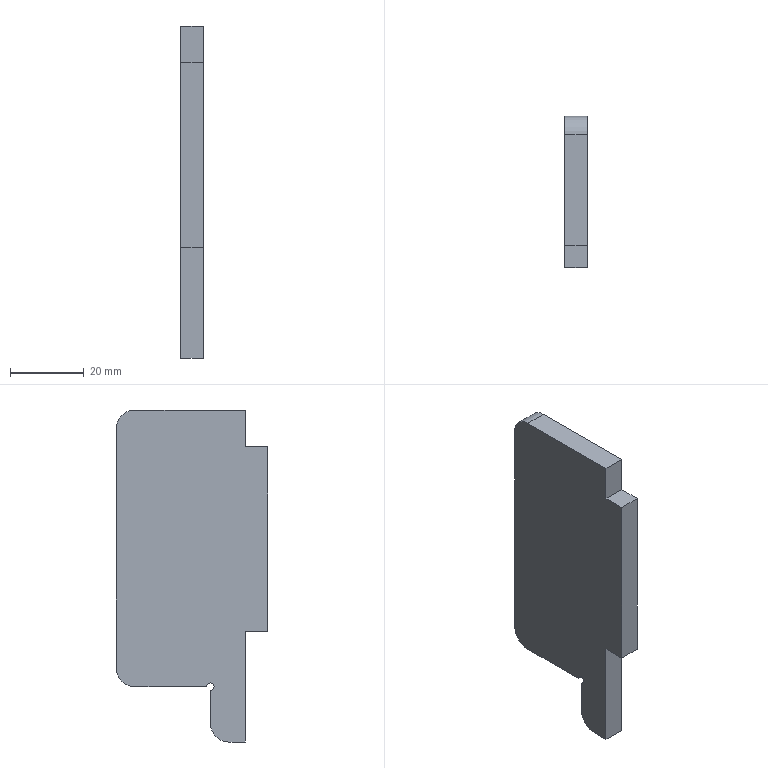Part | SolidWorks | features FlatPattern 1, SMBaseFlange 1, SheetMetal 1 | 1 solid | 16 faces | box 6 x 41 x 90 mm | volume 18294 mm3 | plane 12 | cylinder 4 | commonest cylinder face diameters 10 x3 2 x1
STEP:
#1=CARTESIAN_POINT('',(0.,0.,0.));
#2=VERTEX_POINT('',#1);
#3=CARTESIAN_POINT('',(0.,4.5,0.));
#4=VERTEX_POINT('',#3);
#5=CARTESIAN_POINT('',(0.,4.5,0.));
#6=DIRECTION('',(0.,1.,0.));
#7=VECTOR('',#6,1000.);
#8=LINE('',#5,#7);
#9=EDGE_CURVE('',#2,#4,#8,.T.);
#10=ORIENTED_EDGE('',*,*,#9,.F.);
#11=CARTESIAN_POINT('',(-6.,0.,0.));
#12=VERTEX_POINT('',#11);
#13=CARTESIAN_POINT('',(-6.,0.,0.));
#14=DIRECTION('',(1.,0.,0.));
#15=VECTOR('',#14,1000.);
#16=LINE('',#13,#15);
#17=EDGE_CURVE('',#12,#2,#16,.T.);
#18=ORIENTED_EDGE('',*,*,#17,.F.);
#19=CARTESIAN_POINT('',(-6.,4.5,0.));
#20=VERTEX_POINT('',#19);
#21=CARTESIAN_POINT('',(-6.,4.5,0.));
#22=DIRECTION('',(0.,1.,0.));
#23=VECTOR('',#22,1000.);
#24=LINE('',#21,#23);
#25=EDGE_CURVE('',#12,#20,#24,.T.);
#26=ORIENTED_EDGE('',*,*,#25,.T.);
#27=CARTESIAN_POINT('',(-6.,4.5,0.));
#28=DIRECTION('',(1.,0.,0.));
#29=VECTOR('',#28,1000.);
#30=LINE('',#27,#29);
#31=EDGE_CURVE('',#20,#4,#30,.T.);
#32=ORIENTED_EDGE('',*,*,#31,.T.);
#33=EDGE_LOOP('',(#10,#18,#26,#32));
#34=FACE_OUTER_BOUND('',#33,.T.);
#35=CARTESIAN_POINT('',(-6.,4.5,0.));
#36=DIRECTION('',(0.,0.,-1.));
#37=DIRECTION('',(-1.,0.,0.));
#38=AXIS2_PLACEMENT_3D('',#35,#36,#37);
#39=PLANE('',#38);
#40=ADVANCED_FACE('',(#34),#39,.T.);
#41=CARTESIAN_POINT('',(0.,0.,30.));
#42=VERTEX_POINT('',#41);
#43=CARTESIAN_POINT('',(0.,0.,0.));
#44=DIRECTION('',(0.,0.,-1.));
#45=VECTOR('',#44,1000.);
#46=LINE('',#43,#45);
#47=EDGE_CURVE('',#42,#2,#46,.T.);
#48=ORIENTED_EDGE('',*,*,#47,.F.);
#49=CARTESIAN_POINT('',(-6.,0.,30.));
#50=VERTEX_POINT('',#49);
#51=CARTESIAN_POINT('',(-6.,0.,30.));
#52=DIRECTION('',(1.,0.,0.));
#53=VECTOR('',#52,1000.);
#54=LINE('',#51,#53);
#55=EDGE_CURVE('',#50,#42,#54,.T.);
#56=ORIENTED_EDGE('',*,*,#55,.F.);
#57=CARTESIAN_POINT('',(-6.,0.,0.));
#58=DIRECTION('',(0.,0.,-1.));
#59=VECTOR('',#58,1000.);
#60=LINE('',#57,#59);
#61=EDGE_CURVE('',#50,#12,#60,.T.);
#62=ORIENTED_EDGE('',*,*,#61,.T.);
#63=ORIENTED_EDGE('',*,*,#17,.T.);
#64=EDGE_LOOP('',(#48,#56,#62,#63));
#65=FACE_OUTER_BOUND('',#64,.T.);
#66=CARTESIAN_POINT('',(-6.,0.,0.));
#67=DIRECTION('',(0.,-1.,0.));
#68=DIRECTION('',(0.,0.,-1.));
#69=AXIS2_PLACEMENT_3D('',#66,#67,#68);
#70=PLANE('',#69);
#71=ADVANCED_FACE('',(#65),#70,.T.);
#72=CARTESIAN_POINT('',(0.,-6.,30.));
#73=VERTEX_POINT('',#72);
#74=CARTESIAN_POINT('',(0.,-6.,30.));
#75=DIRECTION('',(0.,1.,0.));
#76=VECTOR('',#75,1000.);
#77=LINE('',#74,#76);
#78=EDGE_CURVE('',#73,#42,#77,.T.);
#79=ORIENTED_EDGE('',*,*,#78,.F.);
#80=CARTESIAN_POINT('',(-6.,-6.,30.));
#81=VERTEX_POINT('',#80);
#82=CARTESIAN_POINT('',(-6.,-6.,30.));
#83=DIRECTION('',(1.,0.,0.));
#84=VECTOR('',#83,1000.);
#85=LINE('',#82,#84);
#86=EDGE_CURVE('',#81,#73,#85,.T.);
#87=ORIENTED_EDGE('',*,*,#86,.F.);
#88=CARTESIAN_POINT('',(-6.,-6.,30.));
#89=DIRECTION('',(0.,1.,0.));
#90=VECTOR('',#89,1000.);
#91=LINE('',#88,#90);
#92=EDGE_CURVE('',#81,#50,#91,.T.);
#93=ORIENTED_EDGE('',*,*,#92,.T.);
#94=ORIENTED_EDGE('',*,*,#55,.T.);
#95=EDGE_LOOP('',(#79,#87,#93,#94));
#96=FACE_OUTER_BOUND('',#95,.T.);
#97=CARTESIAN_POINT('',(-6.,-6.,30.));
#98=DIRECTION('',(0.,0.,-1.));
#99=DIRECTION('',(-1.,0.,0.));
#100=AXIS2_PLACEMENT_3D('',#97,#98,#99);
#101=PLANE('',#100);
#102=ADVANCED_FACE('',(#96),#101,.T.);
#103=CARTESIAN_POINT('',(0.,-6.,80.));
#104=VERTEX_POINT('',#103);
#105=CARTESIAN_POINT('',(0.,-6.,80.));
#106=DIRECTION('',(0.,0.,-1.));
#107=VECTOR('',#106,1000.);
#108=LINE('',#105,#107);
#109=EDGE_CURVE('',#104,#73,#108,.T.);
#110=ORIENTED_EDGE('',*,*,#109,.F.);
#111=CARTESIAN_POINT('',(-6.,-6.,80.));
#112=VERTEX_POINT('',#111);
#113=CARTESIAN_POINT('',(-6.,-6.,80.));
#114=DIRECTION('',(1.,0.,0.));
#115=VECTOR('',#114,1000.);
#116=LINE('',#113,#115);
#117=EDGE_CURVE('',#112,#104,#116,.T.);
#118=ORIENTED_EDGE('',*,*,#117,.F.);
#119=CARTESIAN_POINT('',(-6.,-6.,80.));
#120=DIRECTION('',(0.,0.,-1.));
#121=VECTOR('',#120,1000.);
#122=LINE('',#119,#121);
#123=EDGE_CURVE('',#112,#81,#122,.T.);
#124=ORIENTED_EDGE('',*,*,#123,.T.);
#125=ORIENTED_EDGE('',*,*,#86,.T.);
#126=EDGE_LOOP('',(#110,#118,#124,#125));
#127=FACE_OUTER_BOUND('',#126,.T.);
#128=CARTESIAN_POINT('',(-6.,-6.,80.));
#129=DIRECTION('',(0.,-1.,0.));
#130=DIRECTION('',(0.,0.,-1.));
#131=AXIS2_PLACEMENT_3D('',#128,#129,#130);
#132=PLANE('',#131);
#133=ADVANCED_FACE('',(#127),#132,.T.);
#134=CARTESIAN_POINT('',(0.,0.,80.));
#135=VERTEX_POINT('',#134);
#136=CARTESIAN_POINT('',(0.,0.,80.));
#137=DIRECTION('',(0.,-1.,0.));
#138=VECTOR('',#137,1000.);
#139=LINE('',#136,#138);
#140=EDGE_CURVE('',#135,#104,#139,.T.);
#141=ORIENTED_EDGE('',*,*,#140,.F.);
#142=CARTESIAN_POINT('',(-6.,0.,80.));
#143=VERTEX_POINT('',#142);
#144=CARTESIAN_POINT('',(-6.,0.,80.));
#145=DIRECTION('',(1.,0.,0.));
#146=VECTOR('',#145,1000.);
#147=LINE('',#144,#146);
#148=EDGE_CURVE('',#143,#135,#147,.T.);
#149=ORIENTED_EDGE('',*,*,#148,.F.);
#150=CARTESIAN_POINT('',(-6.,0.,80.));
#151=DIRECTION('',(0.,-1.,0.));
#152=VECTOR('',#151,1000.);
#153=LINE('',#150,#152);
#154=EDGE_CURVE('',#143,#112,#153,.T.);
#155=ORIENTED_EDGE('',*,*,#154,.T.);
#156=ORIENTED_EDGE('',*,*,#117,.T.);
#157=EDGE_LOOP('',(#141,#149,#155,#156));
#158=FACE_OUTER_BOUND('',#157,.T.);
#159=CARTESIAN_POINT('',(-6.,0.,80.));
#160=DIRECTION('',(0.,0.,1.));
#161=DIRECTION('',(1.,0.,0.));
#162=AXIS2_PLACEMENT_3D('',#159,#160,#161);
#163=PLANE('',#162);
#164=ADVANCED_FACE('',(#158),#163,.T.);
#165=CARTESIAN_POINT('',(0.,0.,90.));
#166=VERTEX_POINT('',#165);
#167=CARTESIAN_POINT('',(0.,0.,80.));
#168=DIRECTION('',(0.,0.,-1.));
#169=VECTOR('',#168,1000.);
#170=LINE('',#167,#169);
#171=EDGE_CURVE('',#166,#135,#170,.T.);
#172=ORIENTED_EDGE('',*,*,#171,.F.);
#173=CARTESIAN_POINT('',(-6.,0.,90.));
#174=VERTEX_POINT('',#173);
#175=CARTESIAN_POINT('',(-6.,0.,90.));
#176=DIRECTION('',(1.,0.,0.));
#177=VECTOR('',#176,1000.);
#178=LINE('',#175,#177);
#179=EDGE_CURVE('',#174,#166,#178,.T.);
#180=ORIENTED_EDGE('',*,*,#179,.F.);
#181=CARTESIAN_POINT('',(-6.,0.,80.));
#182=DIRECTION('',(0.,0.,-1.));
#183=VECTOR('',#182,1000.);
#184=LINE('',#181,#183);
#185=EDGE_CURVE('',#174,#143,#184,.T.);
#186=ORIENTED_EDGE('',*,*,#185,.T.);
#187=ORIENTED_EDGE('',*,*,#148,.T.);
#188=EDGE_LOOP('',(#172,#180,#186,#187));
#189=FACE_OUTER_BOUND('',#188,.T.);
#190=CARTESIAN_POINT('',(-6.,0.,80.));
#191=DIRECTION('',(0.,-1.,0.));
#192=DIRECTION('',(0.,0.,-1.));
#193=AXIS2_PLACEMENT_3D('',#190,#191,#192);
#194=PLANE('',#193);
#195=ADVANCED_FACE('',(#189),#194,.T.);
#196=CARTESIAN_POINT('',(0.,30.,90.));
#197=VERTEX_POINT('',#196);
#198=CARTESIAN_POINT('',(0.,0.,90.));
#199=DIRECTION('',(0.,-1.,0.));
#200=VECTOR('',#199,1000.);
#201=LINE('',#198,#200);
#202=EDGE_CURVE('',#197,#166,#201,.T.);
#203=ORIENTED_EDGE('',*,*,#202,.F.);
#204=CARTESIAN_POINT('',(-6.,30.,90.));
#205=VERTEX_POINT('',#204);
#206=CARTESIAN_POINT('',(-6.,30.,90.));
#207=DIRECTION('',(1.,0.,0.));
#208=VECTOR('',#207,1000.);
#209=LINE('',#206,#208);
#210=EDGE_CURVE('',#205,#197,#209,.T.);
#211=ORIENTED_EDGE('',*,*,#210,.F.);
#212=CARTESIAN_POINT('',(-6.,0.,90.));
#213=DIRECTION('',(0.,-1.,0.));
#214=VECTOR('',#213,1000.);
#215=LINE('',#212,#214);
#216=EDGE_CURVE('',#205,#174,#215,.T.);
#217=ORIENTED_EDGE('',*,*,#216,.T.);
#218=ORIENTED_EDGE('',*,*,#179,.T.);
#219=EDGE_LOOP('',(#203,#211,#217,#218));
#220=FACE_OUTER_BOUND('',#219,.T.);
#221=CARTESIAN_POINT('',(-6.,0.,90.));
#222=DIRECTION('',(0.,0.,1.));
#223=DIRECTION('',(1.,0.,0.));
#224=AXIS2_PLACEMENT_3D('',#221,#222,#223);
#225=PLANE('',#224);
#226=ADVANCED_FACE('',(#220),#225,.T.);
#227=CARTESIAN_POINT('',(0.,35.,85.));
#228=VERTEX_POINT('',#227);
#229=CARTESIAN_POINT('',(0.,30.,85.));
#230=DIRECTION('',(1.,0.,0.));
#231=DIRECTION('',(0.,0.,1.));
#232=AXIS2_PLACEMENT_3D('',#229,#230,#231);
#233=CIRCLE('',#232,5.);
#234=EDGE_CURVE('',#228,#197,#233,.T.);
#235=ORIENTED_EDGE('',*,*,#234,.F.);
#236=CARTESIAN_POINT('',(-6.,35.,85.));
#237=VERTEX_POINT('',#236);
#238=CARTESIAN_POINT('',(-6.,35.,85.));
#239=DIRECTION('',(1.,0.,0.));
#240=VECTOR('',#239,1000.);
#241=LINE('',#238,#240);
#242=EDGE_CURVE('',#237,#228,#241,.T.);
#243=ORIENTED_EDGE('',*,*,#242,.F.);
#244=CARTESIAN_POINT('',(-6.,30.,85.));
#245=DIRECTION('',(1.,0.,0.));
#246=DIRECTION('',(0.,0.,1.));
#247=AXIS2_PLACEMENT_3D('',#244,#245,#246);
#248=CIRCLE('',#247,5.);
#249=EDGE_CURVE('',#237,#205,#248,.T.);
#250=ORIENTED_EDGE('',*,*,#249,.T.);
#251=ORIENTED_EDGE('',*,*,#210,.T.);
#252=EDGE_LOOP('',(#235,#243,#250,#251));
#253=FACE_OUTER_BOUND('',#252,.T.);
#254=CARTESIAN_POINT('',(-6.,30.,85.));
#255=DIRECTION('',(1.,0.,0.));
#256=DIRECTION('',(0.,0.,-1.));
#257=AXIS2_PLACEMENT_3D('',#254,#255,#256);
#258=CYLINDRICAL_SURFACE('',#257,5.);
#259=ADVANCED_FACE('',(#253),#258,.T.);
#260=CARTESIAN_POINT('',(0.,35.,20.));
#261=VERTEX_POINT('',#260);
#262=CARTESIAN_POINT('',(0.,35.,85.));
#263=DIRECTION('',(0.,0.,1.));
#264=VECTOR('',#263,1000.);
#265=LINE('',#262,#264);
#266=EDGE_CURVE('',#261,#228,#265,.T.);
#267=ORIENTED_EDGE('',*,*,#266,.F.);
#268=CARTESIAN_POINT('',(-6.,35.,20.));
#269=VERTEX_POINT('',#268);
#270=CARTESIAN_POINT('',(-6.,35.,20.));
#271=DIRECTION('',(1.,0.,0.));
#272=VECTOR('',#271,1000.);
#273=LINE('',#270,#272);
#274=EDGE_CURVE('',#269,#261,#273,.T.);
#275=ORIENTED_EDGE('',*,*,#274,.F.);
#276=CARTESIAN_POINT('',(-6.,35.,85.));
#277=DIRECTION('',(0.,0.,1.));
#278=VECTOR('',#277,1000.);
#279=LINE('',#276,#278);
#280=EDGE_CURVE('',#269,#237,#279,.T.);
#281=ORIENTED_EDGE('',*,*,#280,.T.);
#282=ORIENTED_EDGE('',*,*,#242,.T.);
#283=EDGE_LOOP('',(#267,#275,#281,#282));
#284=FACE_OUTER_BOUND('',#283,.T.);
#285=CARTESIAN_POINT('',(-6.,35.,85.));
#286=DIRECTION('',(0.,1.,0.));
#287=DIRECTION('',(0.,0.,1.));
#288=AXIS2_PLACEMENT_3D('',#285,#286,#287);
#289=PLANE('',#288);
#290=ADVANCED_FACE('',(#284),#289,.T.);
#291=CARTESIAN_POINT('',(0.,30.,15.));
#292=VERTEX_POINT('',#291);
#293=CARTESIAN_POINT('',(0.,30.,20.));
#294=DIRECTION('',(1.,0.,0.));
#295=DIRECTION('',(0.,0.,1.));
#296=AXIS2_PLACEMENT_3D('',#293,#294,#295);
#297=CIRCLE('',#296,5.);
#298=EDGE_CURVE('',#292,#261,#297,.T.);
#299=ORIENTED_EDGE('',*,*,#298,.F.);
#300=CARTESIAN_POINT('',(-6.,30.,15.));
#301=VERTEX_POINT('',#300);
#302=CARTESIAN_POINT('',(-6.,30.,15.));
#303=DIRECTION('',(1.,0.,0.));
#304=VECTOR('',#303,1000.);
#305=LINE('',#302,#304);
#306=EDGE_CURVE('',#301,#292,#305,.T.);
#307=ORIENTED_EDGE('',*,*,#306,.F.);
#308=CARTESIAN_POINT('',(-6.,30.,20.));
#309=DIRECTION('',(1.,0.,0.));
#310=DIRECTION('',(0.,0.,1.));
#311=AXIS2_PLACEMENT_3D('',#308,#309,#310);
#312=CIRCLE('',#311,5.);
#313=EDGE_CURVE('',#301,#269,#312,.T.);
#314=ORIENTED_EDGE('',*,*,#313,.T.);
#315=ORIENTED_EDGE('',*,*,#274,.T.);
#316=EDGE_LOOP('',(#299,#307,#314,#315));
#317=FACE_OUTER_BOUND('',#316,.T.);
#318=CARTESIAN_POINT('',(-6.,30.,20.));
#319=DIRECTION('',(1.,0.,0.));
#320=DIRECTION('',(0.,0.,-1.));
#321=AXIS2_PLACEMENT_3D('',#318,#319,#320);
#322=CYLINDRICAL_SURFACE('',#321,5.);
#323=ADVANCED_FACE('',(#317),#322,.T.);
#324=CARTESIAN_POINT('',(0.,10.5,15.));
#325=VERTEX_POINT('',#324);
#326=CARTESIAN_POINT('',(0.,30.,15.));
#327=DIRECTION('',(0.,1.,0.));
#328=VECTOR('',#327,1000.);
#329=LINE('',#326,#328);
#330=EDGE_CURVE('',#325,#292,#329,.T.);
#331=ORIENTED_EDGE('',*,*,#330,.F.);
#332=CARTESIAN_POINT('',(-6.,10.5,15.));
#333=VERTEX_POINT('',#332);
#334=CARTESIAN_POINT('',(-6.,10.5,15.));
#335=DIRECTION('',(1.,0.,0.));
#336=VECTOR('',#335,1000.);
#337=LINE('',#334,#336);
#338=EDGE_CURVE('',#333,#325,#337,.T.);
#339=ORIENTED_EDGE('',*,*,#338,.F.);
#340=CARTESIAN_POINT('',(-6.,30.,15.));
#341=DIRECTION('',(0.,1.,0.));
#342=VECTOR('',#341,1000.);
#343=LINE('',#340,#342);
#344=EDGE_CURVE('',#333,#301,#343,.T.);
#345=ORIENTED_EDGE('',*,*,#344,.T.);
#346=ORIENTED_EDGE('',*,*,#306,.T.);
#347=EDGE_LOOP('',(#331,#339,#345,#346));
#348=FACE_OUTER_BOUND('',#347,.T.);
#349=CARTESIAN_POINT('',(-6.,30.,15.));
#350=DIRECTION('',(0.,0.,-1.));
#351=DIRECTION('',(0.,1.,0.));
#352=AXIS2_PLACEMENT_3D('',#349,#350,#351);
#353=PLANE('',#352);
#354=ADVANCED_FACE('',(#348),#353,.T.);
#355=CARTESIAN_POINT('',(0.,9.5,14.));
#356=VERTEX_POINT('',#355);
#357=CARTESIAN_POINT('',(0.,9.5,15.));
#358=DIRECTION('',(-1.,0.,0.));
#359=DIRECTION('',(0.,0.,-1.));
#360=AXIS2_PLACEMENT_3D('',#357,#358,#359);
#361=CIRCLE('',#360,1.);
#362=EDGE_CURVE('',#356,#325,#361,.T.);
#363=ORIENTED_EDGE('',*,*,#362,.F.);
#364=CARTESIAN_POINT('',(-6.,9.5,14.));
#365=VERTEX_POINT('',#364);
#366=CARTESIAN_POINT('',(-6.,9.5,14.));
#367=DIRECTION('',(1.,0.,0.));
#368=VECTOR('',#367,1000.);
#369=LINE('',#366,#368);
#370=EDGE_CURVE('',#365,#356,#369,.T.);
#371=ORIENTED_EDGE('',*,*,#370,.F.);
#372=CARTESIAN_POINT('',(-6.,9.5,15.));
#373=DIRECTION('',(-1.,0.,0.));
#374=DIRECTION('',(0.,0.,-1.));
#375=AXIS2_PLACEMENT_3D('',#372,#373,#374);
#376=CIRCLE('',#375,1.);
#377=EDGE_CURVE('',#365,#333,#376,.T.);
#378=ORIENTED_EDGE('',*,*,#377,.T.);
#379=ORIENTED_EDGE('',*,*,#338,.T.);
#380=EDGE_LOOP('',(#363,#371,#378,#379));
#381=FACE_OUTER_BOUND('',#380,.T.);
#382=CARTESIAN_POINT('',(-6.,9.5,15.));
#383=DIRECTION('',(1.,0.,0.));
#384=DIRECTION('',(0.,0.,-1.));
#385=AXIS2_PLACEMENT_3D('',#382,#383,#384);
#386=CYLINDRICAL_SURFACE('',#385,1.);
#387=ADVANCED_FACE('',(#381),#386,.F.);
#388=CARTESIAN_POINT('',(0.,9.5,5.));
#389=VERTEX_POINT('',#388);
#390=CARTESIAN_POINT('',(0.,9.5,14.));
#391=DIRECTION('',(0.,0.,1.));
#392=VECTOR('',#391,1000.);
#393=LINE('',#390,#392);
#394=EDGE_CURVE('',#389,#356,#393,.T.);
#395=ORIENTED_EDGE('',*,*,#394,.F.);
#396=CARTESIAN_POINT('',(-6.,9.5,5.));
#397=VERTEX_POINT('',#396);
#398=CARTESIAN_POINT('',(-6.,9.5,5.));
#399=DIRECTION('',(1.,0.,0.));
#400=VECTOR('',#399,1000.);
#401=LINE('',#398,#400);
#402=EDGE_CURVE('',#397,#389,#401,.T.);
#403=ORIENTED_EDGE('',*,*,#402,.F.);
#404=CARTESIAN_POINT('',(-6.,9.5,14.));
#405=DIRECTION('',(0.,0.,1.));
#406=VECTOR('',#405,1000.);
#407=LINE('',#404,#406);
#408=EDGE_CURVE('',#397,#365,#407,.T.);
#409=ORIENTED_EDGE('',*,*,#408,.T.);
#410=ORIENTED_EDGE('',*,*,#370,.T.);
#411=EDGE_LOOP('',(#395,#403,#409,#410));
#412=FACE_OUTER_BOUND('',#411,.T.);
#413=CARTESIAN_POINT('',(-6.,9.5,14.));
#414=DIRECTION('',(0.,1.,0.));
#415=DIRECTION('',(0.,0.,1.));
#416=AXIS2_PLACEMENT_3D('',#413,#414,#415);
#417=PLANE('',#416);
#418=ADVANCED_FACE('',(#412),#417,.T.);
#419=CARTESIAN_POINT('',(0.,4.5,5.));
#420=DIRECTION('',(1.,0.,0.));
#421=DIRECTION('',(0.,0.,1.));
#422=AXIS2_PLACEMENT_3D('',#419,#420,#421);
#423=CIRCLE('',#422,5.);
#424=EDGE_CURVE('',#4,#389,#423,.T.);
#425=ORIENTED_EDGE('',*,*,#424,.F.);
#426=ORIENTED_EDGE('',*,*,#31,.F.);
#427=CARTESIAN_POINT('',(-6.,4.5,5.));
#428=DIRECTION('',(1.,0.,0.));
#429=DIRECTION('',(0.,0.,1.));
#430=AXIS2_PLACEMENT_3D('',#427,#428,#429);
#431=CIRCLE('',#430,5.);
#432=EDGE_CURVE('',#20,#397,#431,.T.);
#433=ORIENTED_EDGE('',*,*,#432,.T.);
#434=ORIENTED_EDGE('',*,*,#402,.T.);
#435=EDGE_LOOP('',(#425,#426,#433,#434));
#436=FACE_OUTER_BOUND('',#435,.T.);
#437=CARTESIAN_POINT('',(-6.,4.5,5.));
#438=DIRECTION('',(1.,0.,0.));
#439=DIRECTION('',(0.,0.,-1.));
#440=AXIS2_PLACEMENT_3D('',#437,#438,#439);
#441=CYLINDRICAL_SURFACE('',#440,5.);
#442=ADVANCED_FACE('',(#436),#441,.T.);
#443=ORIENTED_EDGE('',*,*,#25,.F.);
#444=ORIENTED_EDGE('',*,*,#61,.F.);
#445=ORIENTED_EDGE('',*,*,#92,.F.);
#446=ORIENTED_EDGE('',*,*,#123,.F.);
#447=ORIENTED_EDGE('',*,*,#154,.F.);
#448=ORIENTED_EDGE('',*,*,#185,.F.);
#449=ORIENTED_EDGE('',*,*,#216,.F.);
#450=ORIENTED_EDGE('',*,*,#249,.F.);
#451=ORIENTED_EDGE('',*,*,#280,.F.);
#452=ORIENTED_EDGE('',*,*,#313,.F.);
#453=ORIENTED_EDGE('',*,*,#344,.F.);
#454=ORIENTED_EDGE('',*,*,#377,.F.);
#455=ORIENTED_EDGE('',*,*,#408,.F.);
#456=ORIENTED_EDGE('',*,*,#432,.F.);
#457=EDGE_LOOP('',(#443,#444,#445,#446,#447,#448,#449,#450,#451,#452,#453,#454,#455,#456));
#458=FACE_OUTER_BOUND('',#457,.T.);
#459=CARTESIAN_POINT('',(-6.,30.,85.));
#460=DIRECTION('',(-1.,0.,0.));
#461=DIRECTION('',(0.,0.,1.));
#462=AXIS2_PLACEMENT_3D('',#459,#460,#461);
#463=PLANE('',#462);
#464=ADVANCED_FACE('',(#458),#463,.T.);
#465=ORIENTED_EDGE('',*,*,#9,.T.);
#466=ORIENTED_EDGE('',*,*,#424,.T.);
#467=ORIENTED_EDGE('',*,*,#394,.T.);
#468=ORIENTED_EDGE('',*,*,#362,.T.);
#469=ORIENTED_EDGE('',*,*,#330,.T.);
#470=ORIENTED_EDGE('',*,*,#298,.T.);
#471=ORIENTED_EDGE('',*,*,#266,.T.);
#472=ORIENTED_EDGE('',*,*,#234,.T.);
#473=ORIENTED_EDGE('',*,*,#202,.T.);
#474=ORIENTED_EDGE('',*,*,#171,.T.);
#475=ORIENTED_EDGE('',*,*,#140,.T.);
#476=ORIENTED_EDGE('',*,*,#109,.T.);
#477=ORIENTED_EDGE('',*,*,#78,.T.);
#478=ORIENTED_EDGE('',*,*,#47,.T.);
#479=EDGE_LOOP('',(#465,#466,#467,#468,#469,#470,#471,#472,#473,#474,#475,#476,#477,#478));
#480=FACE_OUTER_BOUND('',#479,.T.);
#481=CARTESIAN_POINT('',(0.,30.,85.));
#482=DIRECTION('',(-1.,0.,0.));
#483=DIRECTION('',(0.,0.,1.));
#484=AXIS2_PLACEMENT_3D('',#481,#482,#483);
#485=PLANE('',#484);
#486=ADVANCED_FACE('',(#480),#485,.F.);
#487=CLOSED_SHELL('',(#40,#71,#102,#133,#164,#195,#226,#259,#290,#323,#354,#387,#418,#442,#464,#486));
#488=MANIFOLD_SOLID_BREP('',#487);
#489=CARTESIAN_POINT('',(0.,0.,0.));
#490=DIRECTION('',(0.,0.,1.));
#491=DIRECTION('',(1.,0.,0.));
#492=AXIS2_PLACEMENT_3D('',#489,#490,#491);
#493=(LENGTH_UNIT()NAMED_UNIT(*)SI_UNIT(.MILLI.,.METRE.));
#494=UNCERTAINTY_MEASURE_WITH_UNIT(LENGTH_MEASURE(0.00001),#493,'','');
#495=(NAMED_UNIT(*)PLANE_ANGLE_UNIT()SI_UNIT($,.RADIAN.));
#496=(NAMED_UNIT(*)SI_UNIT($,.STERADIAN.)SOLID_ANGLE_UNIT());
#497=(GEOMETRIC_REPRESENTATION_CONTEXT(3)GLOBAL_UNCERTAINTY_ASSIGNED_CONTEXT((#494))GLOBAL_UNIT_ASSIGNED_CONTEXT((#493,#495,#496))REPRESENTATION_CONTEXT('',''));
#498=ADVANCED_BREP_SHAPE_REPRESENTATION('',(#488,#492),#497);